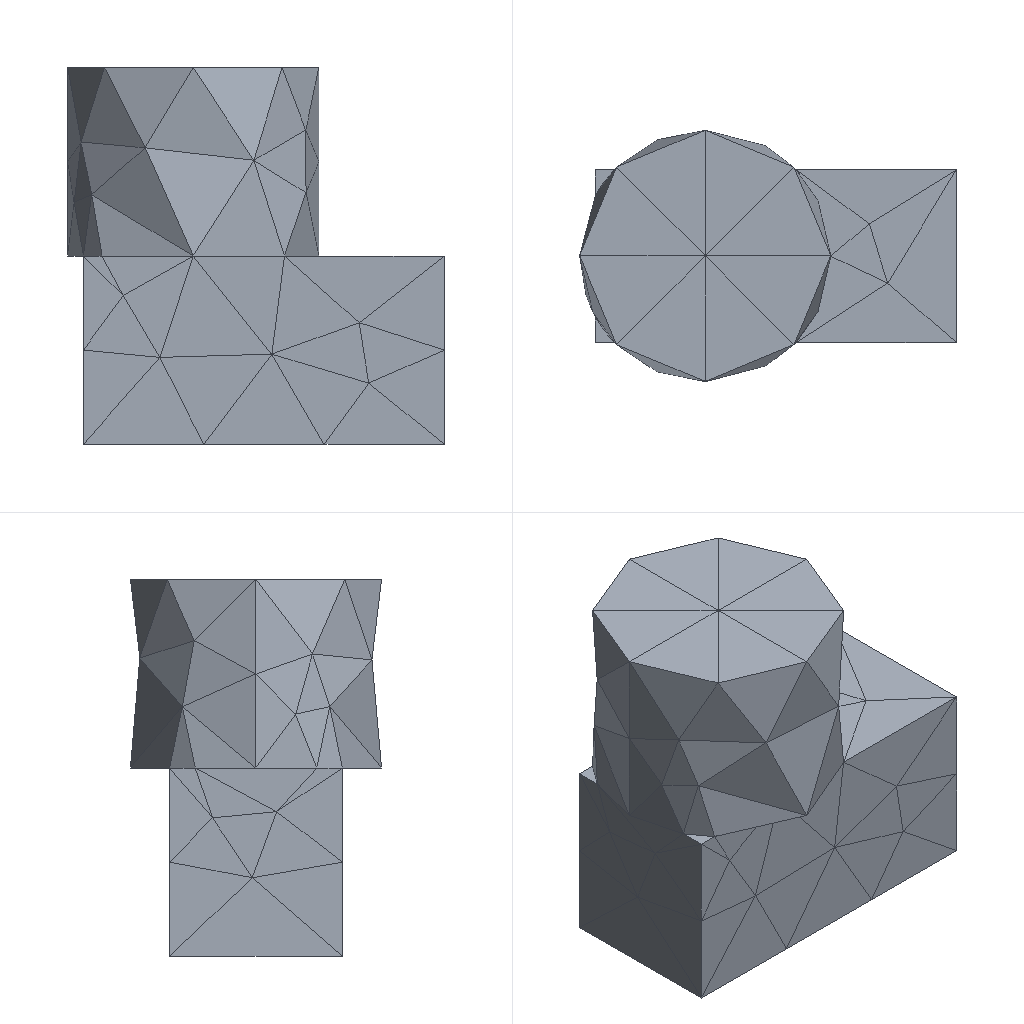Simulation study | ansys mapdl
Set-up summary:
category,name,step,type,value,unit,region
solver,ansys_mapdl
units,mm-N-s-tonne (MPa),,inferred,E=210000 density=
analysis,model,,static
mesh,nodes,,,445
mesh,elements,,,217
element_type,SOLID187,,,217
material,mat 1,,E,210000
material,mat 1,,nu,0.3
load,,model,body load temp,,,all
load,,model,force,"1000 [dir=(0, 0, -1) n=60]",,node list
bc,,model,fixed,"[dofs=UX,UY,UZ n=407]",,node list
Ansys APDL input file, long lists of numbers shortened:
/COM,ANSYS RELEASE 2026 R1           BUILD 26.1      UP20260202       09:10:33
/PREP7
/NOPR
/TITLE,2
ANTYPE, 0
*IF,_CDRDOFF,EQ,1,THEN     !if solid model was read in
_CDRDOFF=             !reset flag, numoffs already performed
*ELSE              !offset database for the following FE model
NUMOFF,NODE,      445
NUMOFF,ELEM,      217
NUMOFF,MAT ,        1
NUMOFF,TYPE,        1
*ENDIF
*SET,_RETURN ,  0.
*SET,_STATUS ,  0.
*SET,_UIQR   ,  60.
*SET,__FLOATPARAMETER__,  445.
DOF,DELETE
ETBLOCK,        1,        1
(2i9,19a9)
        1      187        0        0        0        0        0        0        0        0        0        0        0        0        0        0        0        0        0        0        0
       -1
NBLOCK,6,SOLID,       445,       445
(3i9,6e21.13e3)
        1        0        0 1.1000000000000E+001 1.1000000000000E+001 6.0000000000000E+001
! (444 more lines like these left out)
N,UNBL,LOC,       -1,
EBLOCK,19,SOLID,       217,       217
(19i10)
         1         1         1         1         0         0         0         0        10         0         1       235       231        88       279       212       288       289       290
! (433 more lines like these left out)
        -1
MPTEMP,UNBL, 1, 1,  0.    ,
MPDATA,UNBL, 1,EX  ,       1, 1,  210000.000    ,
MPTEMP,UNBL, 1, 1,  0.    ,
MPDATA,UNBL, 1,NUXY,       1, 1, 0.3    ,
MPTEMP,UNBL, 1, 1,  0.    ,
MPDATA,UNBL, 1,PRXY,       1, 1, 0.3    ,
EXTOPT,ATTR,      0,      0,      0
EXTOPT,ESIZE,  0,  0.
EXTOPT,ACLEAR,      0
TREF,  0.
IRLF,  0
BFUNIF,TEMP,_TINY
ACEL,  0.    ,  0.    ,  0.
OMEGA,  0.    ,  0.    ,  0.
DOMEGA,  0.    ,  0.    ,  0.
CGLOC,  0.    ,  0.    ,  0.
CGOMEGA,  0.    ,  0.    ,  0.
DCGOMG,  0.    ,  0.    ,  0.
KUSE,     0
TIME,  0.
ALPHAD,  0.
BETAD,  0.
DMPRAT,  0.
DMPSTR,  0.
CRPLIM, 0.1    ,   0
CRPLIM,  0.    ,   1
NCNV,     0, 1.000000000E+12,     0,  0.    ,  0.
NEQIT,     0
ERESX,DEFA
DBLOCK,       407
(i9,a6,2(pg16.9))
        1  UX    0.00000000      0.00000000
! (406 more lines like these left out)
       -1
FBLOCK,        60
(i9,a6,2(pg16.9))
      172  FZ   -16.6666667      0.00000000
! (59 more lines like these left out)
       -1
/GO
FINISH
Results summary:
result,analysis_type_db,,,static,unstated
result,n_sets,,,1,unstated
result,load_steps[0].set,load_step=1,,1,unstated
result,load_steps[0].substep,load_step=1,,1,unstated
result,load_steps[0].time,load_step=1,,1,unstated
result,load_steps[0].freq,load_step=1,,1,unstated
result,load_steps[0].max_usum,load_step=1,,0.0006007,unstated
result,load_steps[0].max_seqv,load_step=1,,8.204,unstated
result,load_steps[0].reaction_sum.FX,load_step=1,,-1.1557e-11,unstated
result,load_steps[0].reaction_sum.FY,load_step=1,,1.09708e-11,unstated
result,load_steps[0].reaction_sum.FZ,load_step=1,,1000,unstated
result,load_steps[0].reaction_sum.MX,load_step=1,,0,unstated
result,load_steps[0].reaction_sum.MY,load_step=1,,0,unstated
result,load_steps[0].reaction_sum.MZ,load_step=1,,0,unstated
result,convergence,,,results present for all listed sets,unstated